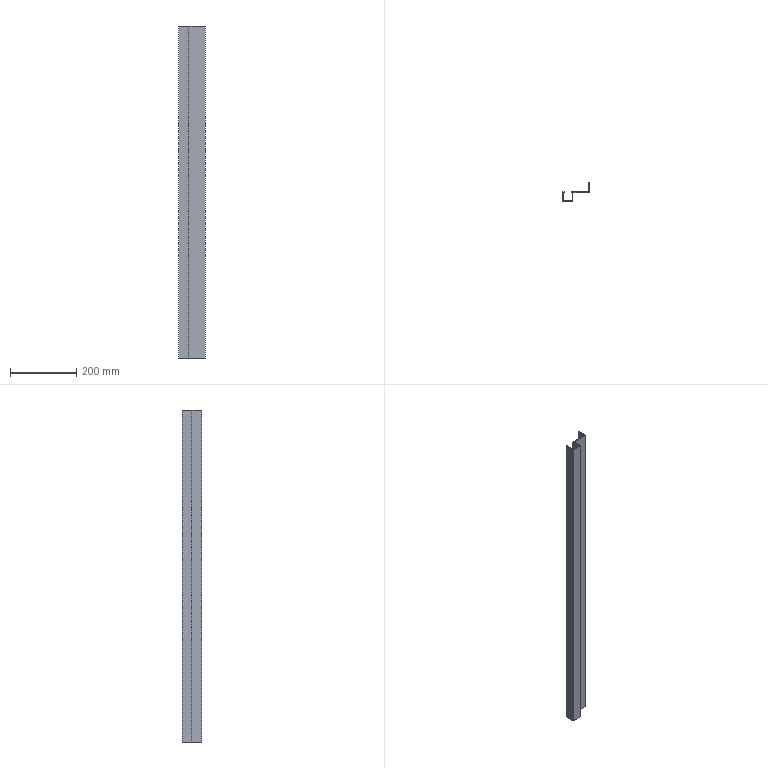Part | STEP file | Rieles_1-22 | 1 solid | 18 faces | box 81.4 x 57.7 x 1003 mm | volume 261332 mm3 | plane 18
STEP:
#1=CARTESIAN_POINT('',(10.,26.2,-551.));
#2=VERTEX_POINT('',#1);
#3=CARTESIAN_POINT('',(10.,27.7,-551.));
#4=VERTEX_POINT('',#3);
#5=CARTESIAN_POINT('',(10.,27.35,-551.));
#6=DIRECTION('',(0.,1.,0.));
#7=VECTOR('',#6,1000.);
#8=LINE('',#5,#7);
#9=EDGE_CURVE('',#2,#4,#8,.T.);
#10=ORIENTED_EDGE('',*,*,#9,.T.);
#11=CARTESIAN_POINT('',(64.2,27.7,-551.));
#12=VERTEX_POINT('',#11);
#13=CARTESIAN_POINT('',(25.,27.7,-551.));
#14=DIRECTION('',(1.,0.,0.));
#15=VECTOR('',#14,1000.);
#16=LINE('',#13,#15);
#17=EDGE_CURVE('',#4,#12,#16,.T.);
#18=ORIENTED_EDGE('',*,*,#17,.T.);
#19=CARTESIAN_POINT('',(64.2,56.2,-551.));
#20=VERTEX_POINT('',#19);
#21=CARTESIAN_POINT('',(64.2,27.35,-551.));
#22=DIRECTION('',(0.,1.,0.));
#23=VECTOR('',#22,1000.);
#24=LINE('',#21,#23);
#25=EDGE_CURVE('',#12,#20,#24,.T.);
#26=ORIENTED_EDGE('',*,*,#25,.T.);
#27=CARTESIAN_POINT('',(65.7,56.2,-551.));
#28=VERTEX_POINT('',#27);
#29=CARTESIAN_POINT('',(25.,56.2,-551.));
#30=DIRECTION('',(1.,0.,0.));
#31=VECTOR('',#30,1000.);
#32=LINE('',#29,#31);
#33=EDGE_CURVE('',#20,#28,#32,.T.);
#34=ORIENTED_EDGE('',*,*,#33,.T.);
#35=CARTESIAN_POINT('',(65.7,26.2,-551.));
#36=VERTEX_POINT('',#35);
#37=CARTESIAN_POINT('',(65.7,27.35,-551.));
#38=DIRECTION('',(0.,-1.,0.));
#39=VECTOR('',#38,1000.);
#40=LINE('',#37,#39);
#41=EDGE_CURVE('',#28,#36,#40,.T.);
#42=ORIENTED_EDGE('',*,*,#41,.T.);
#43=CARTESIAN_POINT('',(15.7,26.2,-551.));
#44=VERTEX_POINT('',#43);
#45=CARTESIAN_POINT('',(25.,26.2,-551.));
#46=DIRECTION('',(-1.,0.,0.));
#47=VECTOR('',#46,1000.);
#48=LINE('',#45,#47);
#49=EDGE_CURVE('',#36,#44,#48,.T.);
#50=ORIENTED_EDGE('',*,*,#49,.T.);
#51=CARTESIAN_POINT('',(15.7,-1.5,-551.));
#52=VERTEX_POINT('',#51);
#53=CARTESIAN_POINT('',(15.7,27.35,-551.));
#54=DIRECTION('',(0.,-1.,0.));
#55=VECTOR('',#54,1000.);
#56=LINE('',#53,#55);
#57=EDGE_CURVE('',#44,#52,#56,.T.);
#58=ORIENTED_EDGE('',*,*,#57,.T.);
#59=CARTESIAN_POINT('',(-15.7,-1.5,-551.));
#60=VERTEX_POINT('',#59);
#61=CARTESIAN_POINT('',(25.,-1.5,-551.));
#62=DIRECTION('',(-1.,0.,0.));
#63=VECTOR('',#62,1000.);
#64=LINE('',#61,#63);
#65=EDGE_CURVE('',#52,#60,#64,.T.);
#66=ORIENTED_EDGE('',*,*,#65,.T.);
#67=CARTESIAN_POINT('',(-15.7,27.7,-551.));
#68=VERTEX_POINT('',#67);
#69=CARTESIAN_POINT('',(-15.7,27.35,-551.));
#70=DIRECTION('',(0.,1.,0.));
#71=VECTOR('',#70,1000.);
#72=LINE('',#69,#71);
#73=EDGE_CURVE('',#60,#68,#72,.T.);
#74=ORIENTED_EDGE('',*,*,#73,.T.);
#75=CARTESIAN_POINT('',(-10.,27.7,-551.));
#76=VERTEX_POINT('',#75);
#77=CARTESIAN_POINT('',(25.,27.7,-551.));
#78=DIRECTION('',(1.,0.,0.));
#79=VECTOR('',#78,1000.);
#80=LINE('',#77,#79);
#81=EDGE_CURVE('',#68,#76,#80,.T.);
#82=ORIENTED_EDGE('',*,*,#81,.T.);
#83=CARTESIAN_POINT('',(-10.,26.2,-551.));
#84=VERTEX_POINT('',#83);
#85=CARTESIAN_POINT('',(-10.,27.35,-551.));
#86=DIRECTION('',(0.,-1.,0.));
#87=VECTOR('',#86,1000.);
#88=LINE('',#85,#87);
#89=EDGE_CURVE('',#76,#84,#88,.T.);
#90=ORIENTED_EDGE('',*,*,#89,.T.);
#91=CARTESIAN_POINT('',(-14.2,26.2,-551.));
#92=VERTEX_POINT('',#91);
#93=CARTESIAN_POINT('',(25.,26.2,-551.));
#94=DIRECTION('',(-1.,0.,0.));
#95=VECTOR('',#94,1000.);
#96=LINE('',#93,#95);
#97=EDGE_CURVE('',#84,#92,#96,.T.);
#98=ORIENTED_EDGE('',*,*,#97,.T.);
#99=CARTESIAN_POINT('',(-14.2,0.,-551.));
#100=VERTEX_POINT('',#99);
#101=CARTESIAN_POINT('',(-14.2,27.35,-551.));
#102=DIRECTION('',(0.,-1.,0.));
#103=VECTOR('',#102,1000.);
#104=LINE('',#101,#103);
#105=EDGE_CURVE('',#92,#100,#104,.T.);
#106=ORIENTED_EDGE('',*,*,#105,.T.);
#107=CARTESIAN_POINT('',(14.2,0.,-551.));
#108=VERTEX_POINT('',#107);
#109=CARTESIAN_POINT('',(25.,0.,-551.));
#110=DIRECTION('',(1.,0.,0.));
#111=VECTOR('',#110,1000.);
#112=LINE('',#109,#111);
#113=EDGE_CURVE('',#100,#108,#112,.T.);
#114=ORIENTED_EDGE('',*,*,#113,.T.);
#115=CARTESIAN_POINT('',(14.2,26.2,-551.));
#116=VERTEX_POINT('',#115);
#117=CARTESIAN_POINT('',(14.2,27.35,-551.));
#118=DIRECTION('',(0.,1.,0.));
#119=VECTOR('',#118,1000.);
#120=LINE('',#117,#119);
#121=EDGE_CURVE('',#108,#116,#120,.T.);
#122=ORIENTED_EDGE('',*,*,#121,.T.);
#123=CARTESIAN_POINT('',(25.,26.2,-551.));
#124=DIRECTION('',(-1.,0.,0.));
#125=VECTOR('',#124,1000.);
#126=LINE('',#123,#125);
#127=EDGE_CURVE('',#116,#2,#126,.T.);
#128=ORIENTED_EDGE('',*,*,#127,.T.);
#129=EDGE_LOOP('',(#10,#18,#26,#34,#42,#50,#58,#66,#74,#82,#90,#98,#106,#114,#122,#128));
#130=FACE_OUTER_BOUND('',#129,.T.);
#131=CARTESIAN_POINT('',(25.,27.35,-551.));
#132=DIRECTION('',(0.,0.,-1.));
#133=DIRECTION('',(0.,-1.,0.));
#134=AXIS2_PLACEMENT_3D('',#131,#132,#133);
#135=PLANE('',#134);
#136=ADVANCED_FACE('',(#130),#135,.T.);
#137=CARTESIAN_POINT('',(10.,26.2,452.));
#138=VERTEX_POINT('',#137);
#139=CARTESIAN_POINT('',(10.,27.7,452.));
#140=VERTEX_POINT('',#139);
#141=CARTESIAN_POINT('',(10.,26.2,452.));
#142=DIRECTION('',(0.,1.,0.));
#143=VECTOR('',#142,1000.);
#144=LINE('',#141,#143);
#145=EDGE_CURVE('',#138,#140,#144,.T.);
#146=ORIENTED_EDGE('',*,*,#145,.F.);
#147=CARTESIAN_POINT('',(14.2,26.2,452.));
#148=VERTEX_POINT('',#147);
#149=CARTESIAN_POINT('',(14.2,26.2,452.));
#150=DIRECTION('',(-1.,0.,0.));
#151=VECTOR('',#150,1000.);
#152=LINE('',#149,#151);
#153=EDGE_CURVE('',#148,#138,#152,.T.);
#154=ORIENTED_EDGE('',*,*,#153,.F.);
#155=CARTESIAN_POINT('',(14.2,0.,452.));
#156=VERTEX_POINT('',#155);
#157=CARTESIAN_POINT('',(14.2,0.,452.));
#158=DIRECTION('',(0.,1.,0.));
#159=VECTOR('',#158,1000.);
#160=LINE('',#157,#159);
#161=EDGE_CURVE('',#156,#148,#160,.T.);
#162=ORIENTED_EDGE('',*,*,#161,.F.);
#163=CARTESIAN_POINT('',(-14.2,0.,452.));
#164=VERTEX_POINT('',#163);
#165=CARTESIAN_POINT('',(-14.2,0.,452.));
#166=DIRECTION('',(1.,0.,0.));
#167=VECTOR('',#166,1000.);
#168=LINE('',#165,#167);
#169=EDGE_CURVE('',#164,#156,#168,.T.);
#170=ORIENTED_EDGE('',*,*,#169,.F.);
#171=CARTESIAN_POINT('',(-14.2,26.2,452.));
#172=VERTEX_POINT('',#171);
#173=CARTESIAN_POINT('',(-14.2,26.2,452.));
#174=DIRECTION('',(0.,-1.,0.));
#175=VECTOR('',#174,1000.);
#176=LINE('',#173,#175);
#177=EDGE_CURVE('',#172,#164,#176,.T.);
#178=ORIENTED_EDGE('',*,*,#177,.F.);
#179=CARTESIAN_POINT('',(-10.,26.2,452.));
#180=VERTEX_POINT('',#179);
#181=CARTESIAN_POINT('',(-10.,26.2,452.));
#182=DIRECTION('',(-1.,0.,0.));
#183=VECTOR('',#182,1000.);
#184=LINE('',#181,#183);
#185=EDGE_CURVE('',#180,#172,#184,.T.);
#186=ORIENTED_EDGE('',*,*,#185,.F.);
#187=CARTESIAN_POINT('',(-10.,27.7,452.));
#188=VERTEX_POINT('',#187);
#189=CARTESIAN_POINT('',(-10.,27.7,452.));
#190=DIRECTION('',(0.,-1.,0.));
#191=VECTOR('',#190,1000.);
#192=LINE('',#189,#191);
#193=EDGE_CURVE('',#188,#180,#192,.T.);
#194=ORIENTED_EDGE('',*,*,#193,.F.);
#195=CARTESIAN_POINT('',(-15.7,27.7,452.));
#196=VERTEX_POINT('',#195);
#197=CARTESIAN_POINT('',(-15.7,27.7,452.));
#198=DIRECTION('',(1.,0.,0.));
#199=VECTOR('',#198,1000.);
#200=LINE('',#197,#199);
#201=EDGE_CURVE('',#196,#188,#200,.T.);
#202=ORIENTED_EDGE('',*,*,#201,.F.);
#203=CARTESIAN_POINT('',(-15.7,-1.5,452.));
#204=VERTEX_POINT('',#203);
#205=CARTESIAN_POINT('',(-15.7,-1.5,452.));
#206=DIRECTION('',(0.,1.,0.));
#207=VECTOR('',#206,1000.);
#208=LINE('',#205,#207);
#209=EDGE_CURVE('',#204,#196,#208,.T.);
#210=ORIENTED_EDGE('',*,*,#209,.F.);
#211=CARTESIAN_POINT('',(15.7,-1.5,452.));
#212=VERTEX_POINT('',#211);
#213=CARTESIAN_POINT('',(15.7,-1.5,452.));
#214=DIRECTION('',(-1.,0.,0.));
#215=VECTOR('',#214,1000.);
#216=LINE('',#213,#215);
#217=EDGE_CURVE('',#212,#204,#216,.T.);
#218=ORIENTED_EDGE('',*,*,#217,.F.);
#219=CARTESIAN_POINT('',(15.7,26.2,452.));
#220=VERTEX_POINT('',#219);
#221=CARTESIAN_POINT('',(15.7,26.2,452.));
#222=DIRECTION('',(0.,-1.,0.));
#223=VECTOR('',#222,1000.);
#224=LINE('',#221,#223);
#225=EDGE_CURVE('',#220,#212,#224,.T.);
#226=ORIENTED_EDGE('',*,*,#225,.F.);
#227=CARTESIAN_POINT('',(65.7,26.2,452.));
#228=VERTEX_POINT('',#227);
#229=CARTESIAN_POINT('',(65.7,26.2,452.));
#230=DIRECTION('',(-1.,0.,0.));
#231=VECTOR('',#230,1000.);
#232=LINE('',#229,#231);
#233=EDGE_CURVE('',#228,#220,#232,.T.);
#234=ORIENTED_EDGE('',*,*,#233,.F.);
#235=CARTESIAN_POINT('',(65.7,56.2,452.));
#236=VERTEX_POINT('',#235);
#237=CARTESIAN_POINT('',(65.7,56.2,452.));
#238=DIRECTION('',(0.,-1.,0.));
#239=VECTOR('',#238,1000.);
#240=LINE('',#237,#239);
#241=EDGE_CURVE('',#236,#228,#240,.T.);
#242=ORIENTED_EDGE('',*,*,#241,.F.);
#243=CARTESIAN_POINT('',(64.2,56.2,452.));
#244=VERTEX_POINT('',#243);
#245=CARTESIAN_POINT('',(64.2,56.2,452.));
#246=DIRECTION('',(1.,0.,0.));
#247=VECTOR('',#246,1000.);
#248=LINE('',#245,#247);
#249=EDGE_CURVE('',#244,#236,#248,.T.);
#250=ORIENTED_EDGE('',*,*,#249,.F.);
#251=CARTESIAN_POINT('',(64.2,27.7,452.));
#252=VERTEX_POINT('',#251);
#253=CARTESIAN_POINT('',(64.2,27.7,452.));
#254=DIRECTION('',(0.,1.,0.));
#255=VECTOR('',#254,1000.);
#256=LINE('',#253,#255);
#257=EDGE_CURVE('',#252,#244,#256,.T.);
#258=ORIENTED_EDGE('',*,*,#257,.F.);
#259=CARTESIAN_POINT('',(10.,27.7,452.));
#260=DIRECTION('',(1.,0.,0.));
#261=VECTOR('',#260,1000.);
#262=LINE('',#259,#261);
#263=EDGE_CURVE('',#140,#252,#262,.T.);
#264=ORIENTED_EDGE('',*,*,#263,.F.);
#265=EDGE_LOOP('',(#146,#154,#162,#170,#178,#186,#194,#202,#210,#218,#226,#234,#242,#250,#258,#264));
#266=FACE_OUTER_BOUND('',#265,.T.);
#267=CARTESIAN_POINT('',(25.,27.35,452.));
#268=DIRECTION('',(0.,0.,1.));
#269=DIRECTION('',(1.,0.,0.));
#270=AXIS2_PLACEMENT_3D('',#267,#268,#269);
#271=PLANE('',#270);
#272=ADVANCED_FACE('',(#266),#271,.T.);
#273=ORIENTED_EDGE('',*,*,#145,.T.);
#274=CARTESIAN_POINT('',(10.,27.7,407.));
#275=DIRECTION('',(0.,0.,-1.));
#276=VECTOR('',#275,1000.);
#277=LINE('',#274,#276);
#278=EDGE_CURVE('',#140,#4,#277,.T.);
#279=ORIENTED_EDGE('',*,*,#278,.T.);
#280=ORIENTED_EDGE('',*,*,#9,.F.);
#281=CARTESIAN_POINT('',(10.,26.2,407.));
#282=DIRECTION('',(0.,0.,-1.));
#283=VECTOR('',#282,1000.);
#284=LINE('',#281,#283);
#285=EDGE_CURVE('',#138,#2,#284,.T.);
#286=ORIENTED_EDGE('',*,*,#285,.F.);
#287=EDGE_LOOP('',(#273,#279,#280,#286));
#288=FACE_OUTER_BOUND('',#287,.T.);
#289=CARTESIAN_POINT('',(10.,26.2,407.));
#290=DIRECTION('',(-1.,0.,0.));
#291=DIRECTION('',(0.,0.,1.));
#292=AXIS2_PLACEMENT_3D('',#289,#290,#291);
#293=PLANE('',#292);
#294=ADVANCED_FACE('',(#288),#293,.T.);
#295=ORIENTED_EDGE('',*,*,#263,.T.);
#296=CARTESIAN_POINT('',(64.2,27.7,407.));
#297=DIRECTION('',(0.,0.,-1.));
#298=VECTOR('',#297,1000.);
#299=LINE('',#296,#298);
#300=EDGE_CURVE('',#252,#12,#299,.T.);
#301=ORIENTED_EDGE('',*,*,#300,.T.);
#302=ORIENTED_EDGE('',*,*,#17,.F.);
#303=ORIENTED_EDGE('',*,*,#278,.F.);
#304=EDGE_LOOP('',(#295,#301,#302,#303));
#305=FACE_OUTER_BOUND('',#304,.T.);
#306=CARTESIAN_POINT('',(10.,27.7,407.));
#307=DIRECTION('',(0.,1.,0.));
#308=DIRECTION('',(1.,0.,0.));
#309=AXIS2_PLACEMENT_3D('',#306,#307,#308);
#310=PLANE('',#309);
#311=ADVANCED_FACE('',(#305),#310,.T.);
#312=ORIENTED_EDGE('',*,*,#257,.T.);
#313=CARTESIAN_POINT('',(64.2,56.2,407.));
#314=DIRECTION('',(0.,0.,-1.));
#315=VECTOR('',#314,1000.);
#316=LINE('',#313,#315);
#317=EDGE_CURVE('',#244,#20,#316,.T.);
#318=ORIENTED_EDGE('',*,*,#317,.T.);
#319=ORIENTED_EDGE('',*,*,#25,.F.);
#320=ORIENTED_EDGE('',*,*,#300,.F.);
#321=EDGE_LOOP('',(#312,#318,#319,#320));
#322=FACE_OUTER_BOUND('',#321,.T.);
#323=CARTESIAN_POINT('',(64.2,27.7,407.));
#324=DIRECTION('',(-1.,0.,0.));
#325=DIRECTION('',(0.,0.,1.));
#326=AXIS2_PLACEMENT_3D('',#323,#324,#325);
#327=PLANE('',#326);
#328=ADVANCED_FACE('',(#322),#327,.T.);
#329=ORIENTED_EDGE('',*,*,#249,.T.);
#330=CARTESIAN_POINT('',(65.7,56.2,407.));
#331=DIRECTION('',(0.,0.,-1.));
#332=VECTOR('',#331,1000.);
#333=LINE('',#330,#332);
#334=EDGE_CURVE('',#236,#28,#333,.T.);
#335=ORIENTED_EDGE('',*,*,#334,.T.);
#336=ORIENTED_EDGE('',*,*,#33,.F.);
#337=ORIENTED_EDGE('',*,*,#317,.F.);
#338=EDGE_LOOP('',(#329,#335,#336,#337));
#339=FACE_OUTER_BOUND('',#338,.T.);
#340=CARTESIAN_POINT('',(64.2,56.2,407.));
#341=DIRECTION('',(0.,1.,0.));
#342=DIRECTION('',(1.,0.,0.));
#343=AXIS2_PLACEMENT_3D('',#340,#341,#342);
#344=PLANE('',#343);
#345=ADVANCED_FACE('',(#339),#344,.T.);
#346=ORIENTED_EDGE('',*,*,#241,.T.);
#347=CARTESIAN_POINT('',(65.7,26.2,407.));
#348=DIRECTION('',(0.,0.,-1.));
#349=VECTOR('',#348,1000.);
#350=LINE('',#347,#349);
#351=EDGE_CURVE('',#228,#36,#350,.T.);
#352=ORIENTED_EDGE('',*,*,#351,.T.);
#353=ORIENTED_EDGE('',*,*,#41,.F.);
#354=ORIENTED_EDGE('',*,*,#334,.F.);
#355=EDGE_LOOP('',(#346,#352,#353,#354));
#356=FACE_OUTER_BOUND('',#355,.T.);
#357=CARTESIAN_POINT('',(65.7,56.2,407.));
#358=DIRECTION('',(1.,0.,0.));
#359=DIRECTION('',(0.,-1.,0.));
#360=AXIS2_PLACEMENT_3D('',#357,#358,#359);
#361=PLANE('',#360);
#362=ADVANCED_FACE('',(#356),#361,.T.);
#363=ORIENTED_EDGE('',*,*,#233,.T.);
#364=CARTESIAN_POINT('',(15.7,26.2,407.));
#365=DIRECTION('',(0.,0.,-1.));
#366=VECTOR('',#365,1000.);
#367=LINE('',#364,#366);
#368=EDGE_CURVE('',#220,#44,#367,.T.);
#369=ORIENTED_EDGE('',*,*,#368,.T.);
#370=ORIENTED_EDGE('',*,*,#49,.F.);
#371=ORIENTED_EDGE('',*,*,#351,.F.);
#372=EDGE_LOOP('',(#363,#369,#370,#371));
#373=FACE_OUTER_BOUND('',#372,.T.);
#374=CARTESIAN_POINT('',(65.7,26.2,407.));
#375=DIRECTION('',(0.,-1.,0.));
#376=DIRECTION('',(0.,0.,-1.));
#377=AXIS2_PLACEMENT_3D('',#374,#375,#376);
#378=PLANE('',#377);
#379=ADVANCED_FACE('',(#373),#378,.T.);
#380=ORIENTED_EDGE('',*,*,#225,.T.);
#381=CARTESIAN_POINT('',(15.7,-1.5,407.));
#382=DIRECTION('',(0.,0.,-1.));
#383=VECTOR('',#382,1000.);
#384=LINE('',#381,#383);
#385=EDGE_CURVE('',#212,#52,#384,.T.);
#386=ORIENTED_EDGE('',*,*,#385,.T.);
#387=ORIENTED_EDGE('',*,*,#57,.F.);
#388=ORIENTED_EDGE('',*,*,#368,.F.);
#389=EDGE_LOOP('',(#380,#386,#387,#388));
#390=FACE_OUTER_BOUND('',#389,.T.);
#391=CARTESIAN_POINT('',(15.7,26.2,407.));
#392=DIRECTION('',(1.,0.,0.));
#393=DIRECTION('',(0.,1.,0.));
#394=AXIS2_PLACEMENT_3D('',#391,#392,#393);
#395=PLANE('',#394);
#396=ADVANCED_FACE('',(#390),#395,.T.);
#397=ORIENTED_EDGE('',*,*,#217,.T.);
#398=CARTESIAN_POINT('',(-15.7,-1.5,407.));
#399=DIRECTION('',(0.,0.,-1.));
#400=VECTOR('',#399,1000.);
#401=LINE('',#398,#400);
#402=EDGE_CURVE('',#204,#60,#401,.T.);
#403=ORIENTED_EDGE('',*,*,#402,.T.);
#404=ORIENTED_EDGE('',*,*,#65,.F.);
#405=ORIENTED_EDGE('',*,*,#385,.F.);
#406=EDGE_LOOP('',(#397,#403,#404,#405));
#407=FACE_OUTER_BOUND('',#406,.T.);
#408=CARTESIAN_POINT('',(15.7,-1.5,407.));
#409=DIRECTION('',(0.,-1.,0.));
#410=DIRECTION('',(0.,0.,-1.));
#411=AXIS2_PLACEMENT_3D('',#408,#409,#410);
#412=PLANE('',#411);
#413=ADVANCED_FACE('',(#407),#412,.T.);
#414=ORIENTED_EDGE('',*,*,#209,.T.);
#415=CARTESIAN_POINT('',(-15.7,27.7,407.));
#416=DIRECTION('',(0.,0.,-1.));
#417=VECTOR('',#416,1000.);
#418=LINE('',#415,#417);
#419=EDGE_CURVE('',#196,#68,#418,.T.);
#420=ORIENTED_EDGE('',*,*,#419,.T.);
#421=ORIENTED_EDGE('',*,*,#73,.F.);
#422=ORIENTED_EDGE('',*,*,#402,.F.);
#423=EDGE_LOOP('',(#414,#420,#421,#422));
#424=FACE_OUTER_BOUND('',#423,.T.);
#425=CARTESIAN_POINT('',(-15.7,-1.5,407.));
#426=DIRECTION('',(-1.,0.,0.));
#427=DIRECTION('',(0.,0.,1.));
#428=AXIS2_PLACEMENT_3D('',#425,#426,#427);
#429=PLANE('',#428);
#430=ADVANCED_FACE('',(#424),#429,.T.);
#431=ORIENTED_EDGE('',*,*,#201,.T.);
#432=CARTESIAN_POINT('',(-10.,27.7,407.));
#433=DIRECTION('',(0.,0.,-1.));
#434=VECTOR('',#433,1000.);
#435=LINE('',#432,#434);
#436=EDGE_CURVE('',#188,#76,#435,.T.);
#437=ORIENTED_EDGE('',*,*,#436,.T.);
#438=ORIENTED_EDGE('',*,*,#81,.F.);
#439=ORIENTED_EDGE('',*,*,#419,.F.);
#440=EDGE_LOOP('',(#431,#437,#438,#439));
#441=FACE_OUTER_BOUND('',#440,.T.);
#442=CARTESIAN_POINT('',(-15.7,27.7,407.));
#443=DIRECTION('',(0.,1.,0.));
#444=DIRECTION('',(1.,0.,0.));
#445=AXIS2_PLACEMENT_3D('',#442,#443,#444);
#446=PLANE('',#445);
#447=ADVANCED_FACE('',(#441),#446,.T.);
#448=ORIENTED_EDGE('',*,*,#193,.T.);
#449=CARTESIAN_POINT('',(-10.,26.2,407.));
#450=DIRECTION('',(0.,0.,-1.));
#451=VECTOR('',#450,1000.);
#452=LINE('',#449,#451);
#453=EDGE_CURVE('',#180,#84,#452,.T.);
#454=ORIENTED_EDGE('',*,*,#453,.T.);
#455=ORIENTED_EDGE('',*,*,#89,.F.);
#456=ORIENTED_EDGE('',*,*,#436,.F.);
#457=EDGE_LOOP('',(#448,#454,#455,#456));
#458=FACE_OUTER_BOUND('',#457,.T.);
#459=CARTESIAN_POINT('',(-10.,27.7,407.));
#460=DIRECTION('',(1.,0.,0.));
#461=DIRECTION('',(0.,1.,0.));
#462=AXIS2_PLACEMENT_3D('',#459,#460,#461);
#463=PLANE('',#462);
#464=ADVANCED_FACE('',(#458),#463,.T.);
#465=ORIENTED_EDGE('',*,*,#185,.T.);
#466=CARTESIAN_POINT('',(-14.2,26.2,407.));
#467=DIRECTION('',(0.,0.,-1.));
#468=VECTOR('',#467,1000.);
#469=LINE('',#466,#468);
#470=EDGE_CURVE('',#172,#92,#469,.T.);
#471=ORIENTED_EDGE('',*,*,#470,.T.);
#472=ORIENTED_EDGE('',*,*,#97,.F.);
#473=ORIENTED_EDGE('',*,*,#453,.F.);
#474=EDGE_LOOP('',(#465,#471,#472,#473));
#475=FACE_OUTER_BOUND('',#474,.T.);
#476=CARTESIAN_POINT('',(-10.,26.2,407.));
#477=DIRECTION('',(0.,-1.,0.));
#478=DIRECTION('',(0.,0.,-1.));
#479=AXIS2_PLACEMENT_3D('',#476,#477,#478);
#480=PLANE('',#479);
#481=ADVANCED_FACE('',(#475),#480,.T.);
#482=ORIENTED_EDGE('',*,*,#177,.T.);
#483=CARTESIAN_POINT('',(-14.2,0.,407.));
#484=DIRECTION('',(0.,0.,-1.));
#485=VECTOR('',#484,1000.);
#486=LINE('',#483,#485);
#487=EDGE_CURVE('',#164,#100,#486,.T.);
#488=ORIENTED_EDGE('',*,*,#487,.T.);
#489=ORIENTED_EDGE('',*,*,#105,.F.);
#490=ORIENTED_EDGE('',*,*,#470,.F.);
#491=EDGE_LOOP('',(#482,#488,#489,#490));
#492=FACE_OUTER_BOUND('',#491,.T.);
#493=CARTESIAN_POINT('',(-14.2,26.2,407.));
#494=DIRECTION('',(1.,0.,0.));
#495=DIRECTION('',(0.,1.,0.));
#496=AXIS2_PLACEMENT_3D('',#493,#494,#495);
#497=PLANE('',#496);
#498=ADVANCED_FACE('',(#492),#497,.T.);
#499=ORIENTED_EDGE('',*,*,#169,.T.);
#500=CARTESIAN_POINT('',(14.2,0.,407.));
#501=DIRECTION('',(0.,0.,-1.));
#502=VECTOR('',#501,1000.);
#503=LINE('',#500,#502);
#504=EDGE_CURVE('',#156,#108,#503,.T.);
#505=ORIENTED_EDGE('',*,*,#504,.T.);
#506=ORIENTED_EDGE('',*,*,#113,.F.);
#507=ORIENTED_EDGE('',*,*,#487,.F.);
#508=EDGE_LOOP('',(#499,#505,#506,#507));
#509=FACE_OUTER_BOUND('',#508,.T.);
#510=CARTESIAN_POINT('',(-14.2,0.,407.));
#511=DIRECTION('',(0.,1.,0.));
#512=DIRECTION('',(1.,0.,0.));
#513=AXIS2_PLACEMENT_3D('',#510,#511,#512);
#514=PLANE('',#513);
#515=ADVANCED_FACE('',(#509),#514,.T.);
#516=ORIENTED_EDGE('',*,*,#161,.T.);
#517=CARTESIAN_POINT('',(14.2,26.2,407.));
#518=DIRECTION('',(0.,0.,-1.));
#519=VECTOR('',#518,1000.);
#520=LINE('',#517,#519);
#521=EDGE_CURVE('',#148,#116,#520,.T.);
#522=ORIENTED_EDGE('',*,*,#521,.T.);
#523=ORIENTED_EDGE('',*,*,#121,.F.);
#524=ORIENTED_EDGE('',*,*,#504,.F.);
#525=EDGE_LOOP('',(#516,#522,#523,#524));
#526=FACE_OUTER_BOUND('',#525,.T.);
#527=CARTESIAN_POINT('',(14.2,0.,407.));
#528=DIRECTION('',(-1.,0.,0.));
#529=DIRECTION('',(0.,0.,1.));
#530=AXIS2_PLACEMENT_3D('',#527,#528,#529);
#531=PLANE('',#530);
#532=ADVANCED_FACE('',(#526),#531,.T.);
#533=ORIENTED_EDGE('',*,*,#153,.T.);
#534=ORIENTED_EDGE('',*,*,#285,.T.);
#535=ORIENTED_EDGE('',*,*,#127,.F.);
#536=ORIENTED_EDGE('',*,*,#521,.F.);
#537=EDGE_LOOP('',(#533,#534,#535,#536));
#538=FACE_OUTER_BOUND('',#537,.T.);
#539=CARTESIAN_POINT('',(14.2,26.2,407.));
#540=DIRECTION('',(0.,-1.,0.));
#541=DIRECTION('',(-1.,0.,0.));
#542=AXIS2_PLACEMENT_3D('',#539,#540,#541);
#543=PLANE('',#542);
#544=ADVANCED_FACE('',(#538),#543,.T.);
#545=CLOSED_SHELL('',(#136,#272,#294,#311,#328,#345,#362,#379,#396,#413,#430,#447,#464,#481,#498,#515,#532,#544));
#546=MANIFOLD_SOLID_BREP('',#545);
#547=CARTESIAN_POINT('',(0.,0.,0.));
#548=DIRECTION('',(0.,0.,1.));
#549=DIRECTION('',(1.,0.,0.));
#550=AXIS2_PLACEMENT_3D('',#547,#548,#549);
#551=(LENGTH_UNIT()NAMED_UNIT(*)SI_UNIT(.MILLI.,.METRE.));
#552=UNCERTAINTY_MEASURE_WITH_UNIT(LENGTH_MEASURE(0.00001),#551,'','');
#553=(NAMED_UNIT(*)PLANE_ANGLE_UNIT()SI_UNIT($,.RADIAN.));
#554=(NAMED_UNIT(*)SI_UNIT($,.STERADIAN.)SOLID_ANGLE_UNIT());
#555=(GEOMETRIC_REPRESENTATION_CONTEXT(3)GLOBAL_UNCERTAINTY_ASSIGNED_CONTEXT((#552))GLOBAL_UNIT_ASSIGNED_CONTEXT((#551,#553,#554))REPRESENTATION_CONTEXT('',''));
#556=ADVANCED_BREP_SHAPE_REPRESENTATION('',(#546,#550),#555);